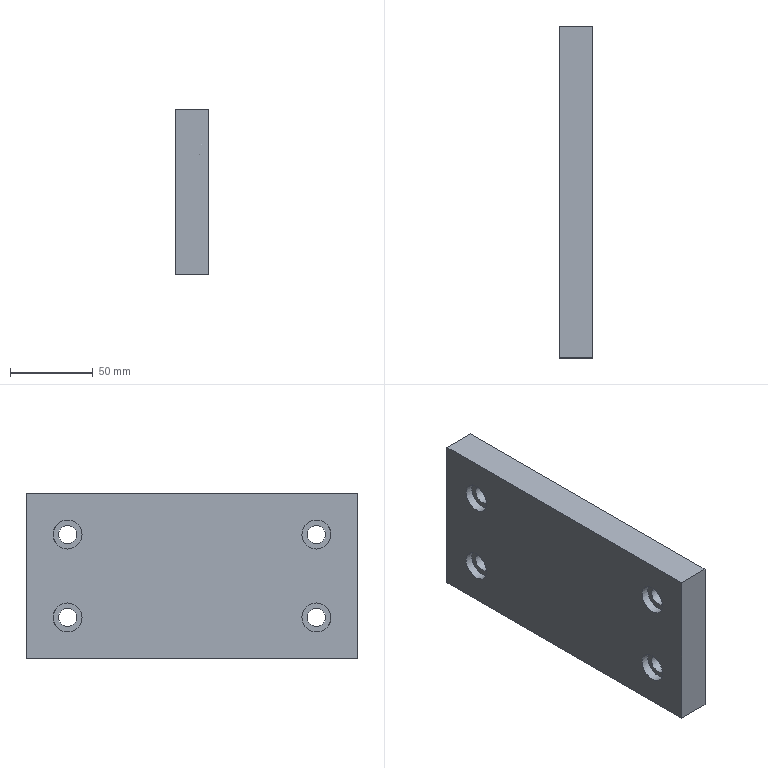Part | NX | features solid 2 | 1 solid | 18 faces | box 20 x 200 x 100 mm | volume 389487 mm3 | plane 10 | cylinder 8 | commonest cylinder face diameters 11 x4 17.5 x4
STEP:
#1=CARTESIAN_POINT('',(-605.,715.,-162.));
#2=VERTEX_POINT('',#1);
#3=CARTESIAN_POINT('',(-605.,715.,-262.));
#4=VERTEX_POINT('',#3);
#5=CARTESIAN_POINT('',(-605.,715.,-160.));
#6=DIRECTION('',(0.,0.,-1.));
#7=VECTOR('',#6,1000.);
#8=LINE('',#5,#7);
#9=EDGE_CURVE('',#2,#4,#8,.T.);
#10=ORIENTED_EDGE('',*,*,#9,.F.);
#11=CARTESIAN_POINT('',(-625.,715.,-162.));
#12=VERTEX_POINT('',#11);
#13=CARTESIAN_POINT('',(-615.,715.,-162.));
#14=DIRECTION('',(1.,0.,0.));
#15=VECTOR('',#14,1000.);
#16=LINE('',#13,#15);
#17=EDGE_CURVE('',#12,#2,#16,.T.);
#18=ORIENTED_EDGE('',*,*,#17,.F.);
#19=CARTESIAN_POINT('',(-625.,715.,-262.));
#20=VERTEX_POINT('',#19);
#21=CARTESIAN_POINT('',(-625.,715.,-160.));
#22=DIRECTION('',(0.,0.,1.));
#23=VECTOR('',#22,1000.);
#24=LINE('',#21,#23);
#25=EDGE_CURVE('',#20,#12,#24,.T.);
#26=ORIENTED_EDGE('',*,*,#25,.F.);
#27=CARTESIAN_POINT('',(-615.,715.,-262.));
#28=DIRECTION('',(1.,0.,0.));
#29=VECTOR('',#28,1000.);
#30=LINE('',#27,#29);
#31=EDGE_CURVE('',#20,#4,#30,.T.);
#32=ORIENTED_EDGE('',*,*,#31,.T.);
#33=EDGE_LOOP('',(#10,#18,#26,#32));
#34=FACE_BOUND('',#33,.T.);
#35=CARTESIAN_POINT('',(-615.,715.,-160.));
#36=DIRECTION('',(0.,-1.,0.));
#37=DIRECTION('',(-1.,0.,0.));
#38=AXIS2_PLACEMENT_3D('',#35,#36,#37);
#39=PLANE('',#38);
#40=ADVANCED_FACE('',(#34),#39,.T.);
#41=CARTESIAN_POINT('',(-605.,740.,-192.5));
#42=VERTEX_POINT('',#41);
#43=CARTESIAN_POINT('',(-605.,740.,-187.));
#44=DIRECTION('',(1.,0.,0.));
#45=DIRECTION('',(0.,0.,-1.));
#46=AXIS2_PLACEMENT_3D('',#43,#44,#45);
#47=CIRCLE('',#46,5.5);
#48=EDGE_CURVE('',#42,#42,#47,.F.);
#49=ORIENTED_EDGE('',*,*,#48,.T.);
#50=EDGE_LOOP('',(#49));
#51=FACE_BOUND('',#50,.T.);
#52=CARTESIAN_POINT('',(-605.,890.,-192.5));
#53=VERTEX_POINT('',#52);
#54=CARTESIAN_POINT('',(-605.,890.,-187.));
#55=DIRECTION('',(1.,0.,0.));
#56=DIRECTION('',(0.,0.,-1.));
#57=AXIS2_PLACEMENT_3D('',#54,#55,#56);
#58=CIRCLE('',#57,5.5);
#59=EDGE_CURVE('',#53,#53,#58,.F.);
#60=ORIENTED_EDGE('',*,*,#59,.T.);
#61=EDGE_LOOP('',(#60));
#62=FACE_BOUND('',#61,.T.);
#63=CARTESIAN_POINT('',(-605.,915.,-262.));
#64=VERTEX_POINT('',#63);
#65=CARTESIAN_POINT('',(-605.,915.,-162.));
#66=VERTEX_POINT('',#65);
#67=CARTESIAN_POINT('',(-605.,915.,-160.));
#68=DIRECTION('',(0.,0.,1.));
#69=VECTOR('',#68,1000.);
#70=LINE('',#67,#69);
#71=EDGE_CURVE('',#64,#66,#70,.T.);
#72=ORIENTED_EDGE('',*,*,#71,.T.);
#73=CARTESIAN_POINT('',(-605.,890.,-162.));
#74=DIRECTION('',(0.,1.,0.));
#75=VECTOR('',#74,1000.);
#76=LINE('',#73,#75);
#77=EDGE_CURVE('',#2,#66,#76,.T.);
#78=ORIENTED_EDGE('',*,*,#77,.F.);
#79=ORIENTED_EDGE('',*,*,#9,.T.);
#80=CARTESIAN_POINT('',(-605.,890.,-262.));
#81=DIRECTION('',(0.,1.,0.));
#82=VECTOR('',#81,1000.);
#83=LINE('',#80,#82);
#84=EDGE_CURVE('',#4,#64,#83,.T.);
#85=ORIENTED_EDGE('',*,*,#84,.T.);
#86=EDGE_LOOP('',(#72,#78,#79,#85));
#87=FACE_BOUND('',#86,.T.);
#88=CARTESIAN_POINT('',(-605.,740.,-231.5));
#89=VERTEX_POINT('',#88);
#90=CARTESIAN_POINT('',(-605.,740.,-237.));
#91=DIRECTION('',(-1.,0.,0.));
#92=DIRECTION('',(0.,0.,1.));
#93=AXIS2_PLACEMENT_3D('',#90,#91,#92);
#94=CIRCLE('',#93,5.5);
#95=EDGE_CURVE('',#89,#89,#94,.F.);
#96=ORIENTED_EDGE('',*,*,#95,.F.);
#97=EDGE_LOOP('',(#96));
#98=FACE_BOUND('',#97,.T.);
#99=CARTESIAN_POINT('',(-605.,890.,-231.5));
#100=VERTEX_POINT('',#99);
#101=CARTESIAN_POINT('',(-605.,890.,-237.));
#102=DIRECTION('',(-1.,0.,0.));
#103=DIRECTION('',(0.,0.,1.));
#104=AXIS2_PLACEMENT_3D('',#101,#102,#103);
#105=CIRCLE('',#104,5.5);
#106=EDGE_CURVE('',#100,#100,#105,.F.);
#107=ORIENTED_EDGE('',*,*,#106,.F.);
#108=EDGE_LOOP('',(#107));
#109=FACE_BOUND('',#108,.T.);
#110=CARTESIAN_POINT('',(-605.,890.,-160.));
#111=DIRECTION('',(1.,0.,0.));
#112=DIRECTION('',(0.,-1.,0.));
#113=AXIS2_PLACEMENT_3D('',#110,#111,#112);
#114=PLANE('',#113);
#115=ADVANCED_FACE('',(#51,#62,#87,#98,#109),#114,.T.);
#116=CARTESIAN_POINT('',(-625.,915.,-162.));
#117=VERTEX_POINT('',#116);
#118=CARTESIAN_POINT('',(-625.,915.,-262.));
#119=VERTEX_POINT('',#118);
#120=CARTESIAN_POINT('',(-625.,915.,-160.));
#121=DIRECTION('',(0.,0.,-1.));
#122=VECTOR('',#121,1000.);
#123=LINE('',#120,#122);
#124=EDGE_CURVE('',#117,#119,#123,.T.);
#125=ORIENTED_EDGE('',*,*,#124,.F.);
#126=CARTESIAN_POINT('',(-615.,915.,-162.));
#127=DIRECTION('',(-1.,0.,0.));
#128=VECTOR('',#127,1000.);
#129=LINE('',#126,#128);
#130=EDGE_CURVE('',#66,#117,#129,.T.);
#131=ORIENTED_EDGE('',*,*,#130,.F.);
#132=ORIENTED_EDGE('',*,*,#71,.F.);
#133=CARTESIAN_POINT('',(-615.,915.,-262.));
#134=DIRECTION('',(-1.,0.,0.));
#135=VECTOR('',#134,1000.);
#136=LINE('',#133,#135);
#137=EDGE_CURVE('',#64,#119,#136,.T.);
#138=ORIENTED_EDGE('',*,*,#137,.T.);
#139=EDGE_LOOP('',(#125,#131,#132,#138));
#140=FACE_BOUND('',#139,.T.);
#141=CARTESIAN_POINT('',(-615.,915.,-160.));
#142=DIRECTION('',(0.,1.,0.));
#143=DIRECTION('',(1.,0.,0.));
#144=AXIS2_PLACEMENT_3D('',#141,#142,#143);
#145=PLANE('',#144);
#146=ADVANCED_FACE('',(#140),#145,.T.);
#147=CARTESIAN_POINT('',(-625.,731.25,-187.));
#148=VERTEX_POINT('',#147);
#149=CARTESIAN_POINT('',(-625.,740.,-187.));
#150=DIRECTION('',(1.,0.,0.));
#151=DIRECTION('',(0.,-1.,0.));
#152=AXIS2_PLACEMENT_3D('',#149,#150,#151);
#153=CIRCLE('',#152,8.75);
#154=EDGE_CURVE('',#148,#148,#153,.T.);
#155=ORIENTED_EDGE('',*,*,#154,.T.);
#156=EDGE_LOOP('',(#155));
#157=FACE_BOUND('',#156,.T.);
#158=CARTESIAN_POINT('',(-625.,881.25,-187.));
#159=VERTEX_POINT('',#158);
#160=CARTESIAN_POINT('',(-625.,890.,-187.));
#161=DIRECTION('',(1.,0.,0.));
#162=DIRECTION('',(0.,-1.,0.));
#163=AXIS2_PLACEMENT_3D('',#160,#161,#162);
#164=CIRCLE('',#163,8.75);
#165=EDGE_CURVE('',#159,#159,#164,.T.);
#166=ORIENTED_EDGE('',*,*,#165,.T.);
#167=EDGE_LOOP('',(#166));
#168=FACE_BOUND('',#167,.T.);
#169=ORIENTED_EDGE('',*,*,#25,.T.);
#170=CARTESIAN_POINT('',(-625.,890.,-162.));
#171=DIRECTION('',(0.,-1.,0.));
#172=VECTOR('',#171,1000.);
#173=LINE('',#170,#172);
#174=EDGE_CURVE('',#117,#12,#173,.T.);
#175=ORIENTED_EDGE('',*,*,#174,.F.);
#176=ORIENTED_EDGE('',*,*,#124,.T.);
#177=CARTESIAN_POINT('',(-625.,890.,-262.));
#178=DIRECTION('',(0.,-1.,0.));
#179=VECTOR('',#178,1000.);
#180=LINE('',#177,#179);
#181=EDGE_CURVE('',#119,#20,#180,.T.);
#182=ORIENTED_EDGE('',*,*,#181,.T.);
#183=EDGE_LOOP('',(#169,#175,#176,#182));
#184=FACE_BOUND('',#183,.T.);
#185=CARTESIAN_POINT('',(-625.,731.25,-237.));
#186=VERTEX_POINT('',#185);
#187=CARTESIAN_POINT('',(-625.,740.,-237.));
#188=DIRECTION('',(-1.,0.,0.));
#189=DIRECTION('',(0.,-1.,0.));
#190=AXIS2_PLACEMENT_3D('',#187,#188,#189);
#191=CIRCLE('',#190,8.75);
#192=EDGE_CURVE('',#186,#186,#191,.T.);
#193=ORIENTED_EDGE('',*,*,#192,.F.);
#194=EDGE_LOOP('',(#193));
#195=FACE_BOUND('',#194,.T.);
#196=CARTESIAN_POINT('',(-625.,881.25,-237.));
#197=VERTEX_POINT('',#196);
#198=CARTESIAN_POINT('',(-625.,890.,-237.));
#199=DIRECTION('',(-1.,0.,0.));
#200=DIRECTION('',(0.,-1.,0.));
#201=AXIS2_PLACEMENT_3D('',#198,#199,#200);
#202=CIRCLE('',#201,8.75);
#203=EDGE_CURVE('',#197,#197,#202,.T.);
#204=ORIENTED_EDGE('',*,*,#203,.F.);
#205=EDGE_LOOP('',(#204));
#206=FACE_BOUND('',#205,.T.);
#207=CARTESIAN_POINT('',(-625.,890.,-160.));
#208=DIRECTION('',(-1.,0.,0.));
#209=DIRECTION('',(0.,1.,0.));
#210=AXIS2_PLACEMENT_3D('',#207,#208,#209);
#211=PLANE('',#210);
#212=ADVANCED_FACE('',(#157,#168,#184,#195,#206),#211,.T.);
#213=CARTESIAN_POINT('',(-620.,740.,-192.5));
#214=VERTEX_POINT('',#213);
#215=CARTESIAN_POINT('',(-620.,740.,-187.));
#216=DIRECTION('',(1.,0.,0.));
#217=DIRECTION('',(0.,0.,-1.));
#218=AXIS2_PLACEMENT_3D('',#215,#216,#217);
#219=CIRCLE('',#218,5.5);
#220=EDGE_CURVE('',#214,#214,#219,.F.);
#221=ORIENTED_EDGE('',*,*,#220,.T.);
#222=EDGE_LOOP('',(#221));
#223=FACE_BOUND('',#222,.T.);
#224=ORIENTED_EDGE('',*,*,#48,.F.);
#225=EDGE_LOOP('',(#224));
#226=FACE_BOUND('',#225,.T.);
#227=CARTESIAN_POINT('',(-605.,740.,-187.));
#228=DIRECTION('',(-1.,0.,0.));
#229=DIRECTION('',(0.,1.,0.));
#230=AXIS2_PLACEMENT_3D('',#227,#228,#229);
#231=CYLINDRICAL_SURFACE('',#230,5.5);
#232=ADVANCED_FACE('',(#223,#226),#231,.F.);
#233=CARTESIAN_POINT('',(-620.,740.,-195.75));
#234=VERTEX_POINT('',#233);
#235=CARTESIAN_POINT('',(-620.,740.,-187.));
#236=DIRECTION('',(1.,0.,0.));
#237=DIRECTION('',(0.,0.,-1.));
#238=AXIS2_PLACEMENT_3D('',#235,#236,#237);
#239=CIRCLE('',#238,8.75);
#240=EDGE_CURVE('',#234,#234,#239,.F.);
#241=ORIENTED_EDGE('',*,*,#240,.T.);
#242=EDGE_LOOP('',(#241));
#243=FACE_BOUND('',#242,.T.);
#244=ORIENTED_EDGE('',*,*,#220,.F.);
#245=EDGE_LOOP('',(#244));
#246=FACE_BOUND('',#245,.T.);
#247=CARTESIAN_POINT('',(-620.,740.,-187.));
#248=DIRECTION('',(1.,0.,0.));
#249=DIRECTION('',(0.,-1.,0.));
#250=AXIS2_PLACEMENT_3D('',#247,#248,#249);
#251=PLANE('',#250);
#252=ADVANCED_FACE('',(#243,#246),#251,.F.);
#253=ORIENTED_EDGE('',*,*,#154,.F.);
#254=EDGE_LOOP('',(#253));
#255=FACE_BOUND('',#254,.T.);
#256=ORIENTED_EDGE('',*,*,#240,.F.);
#257=EDGE_LOOP('',(#256));
#258=FACE_BOUND('',#257,.T.);
#259=CARTESIAN_POINT('',(-610.,740.,-187.));
#260=DIRECTION('',(-1.,0.,0.));
#261=DIRECTION('',(0.,1.,0.));
#262=AXIS2_PLACEMENT_3D('',#259,#260,#261);
#263=CYLINDRICAL_SURFACE('',#262,8.75);
#264=ADVANCED_FACE('',(#255,#258),#263,.F.);
#265=CARTESIAN_POINT('',(-620.,890.,-192.5));
#266=VERTEX_POINT('',#265);
#267=CARTESIAN_POINT('',(-620.,890.,-187.));
#268=DIRECTION('',(1.,0.,0.));
#269=DIRECTION('',(0.,0.,-1.));
#270=AXIS2_PLACEMENT_3D('',#267,#268,#269);
#271=CIRCLE('',#270,5.5);
#272=EDGE_CURVE('',#266,#266,#271,.F.);
#273=ORIENTED_EDGE('',*,*,#272,.T.);
#274=EDGE_LOOP('',(#273));
#275=FACE_BOUND('',#274,.T.);
#276=ORIENTED_EDGE('',*,*,#59,.F.);
#277=EDGE_LOOP('',(#276));
#278=FACE_BOUND('',#277,.T.);
#279=CARTESIAN_POINT('',(-605.,890.,-187.));
#280=DIRECTION('',(-1.,0.,0.));
#281=DIRECTION('',(0.,1.,0.));
#282=AXIS2_PLACEMENT_3D('',#279,#280,#281);
#283=CYLINDRICAL_SURFACE('',#282,5.5);
#284=ADVANCED_FACE('',(#275,#278),#283,.F.);
#285=CARTESIAN_POINT('',(-620.,890.,-195.75));
#286=VERTEX_POINT('',#285);
#287=CARTESIAN_POINT('',(-620.,890.,-187.));
#288=DIRECTION('',(1.,0.,0.));
#289=DIRECTION('',(0.,0.,-1.));
#290=AXIS2_PLACEMENT_3D('',#287,#288,#289);
#291=CIRCLE('',#290,8.75);
#292=EDGE_CURVE('',#286,#286,#291,.F.);
#293=ORIENTED_EDGE('',*,*,#292,.T.);
#294=EDGE_LOOP('',(#293));
#295=FACE_BOUND('',#294,.T.);
#296=ORIENTED_EDGE('',*,*,#272,.F.);
#297=EDGE_LOOP('',(#296));
#298=FACE_BOUND('',#297,.T.);
#299=CARTESIAN_POINT('',(-620.,890.,-187.));
#300=DIRECTION('',(1.,0.,0.));
#301=DIRECTION('',(0.,-1.,0.));
#302=AXIS2_PLACEMENT_3D('',#299,#300,#301);
#303=PLANE('',#302);
#304=ADVANCED_FACE('',(#295,#298),#303,.F.);
#305=ORIENTED_EDGE('',*,*,#165,.F.);
#306=EDGE_LOOP('',(#305));
#307=FACE_BOUND('',#306,.T.);
#308=ORIENTED_EDGE('',*,*,#292,.F.);
#309=EDGE_LOOP('',(#308));
#310=FACE_BOUND('',#309,.T.);
#311=CARTESIAN_POINT('',(-610.,890.,-187.));
#312=DIRECTION('',(-1.,0.,0.));
#313=DIRECTION('',(0.,1.,0.));
#314=AXIS2_PLACEMENT_3D('',#311,#312,#313);
#315=CYLINDRICAL_SURFACE('',#314,8.75);
#316=ADVANCED_FACE('',(#307,#310),#315,.F.);
#317=ORIENTED_EDGE('',*,*,#17,.T.);
#318=ORIENTED_EDGE('',*,*,#77,.T.);
#319=ORIENTED_EDGE('',*,*,#130,.T.);
#320=ORIENTED_EDGE('',*,*,#174,.T.);
#321=EDGE_LOOP('',(#317,#318,#319,#320));
#322=FACE_BOUND('',#321,.T.);
#323=CARTESIAN_POINT('',(-605.,640.,-162.));
#324=DIRECTION('',(0.,0.,-1.));
#325=DIRECTION('',(-1.,0.,0.));
#326=AXIS2_PLACEMENT_3D('',#323,#324,#325);
#327=PLANE('',#326);
#328=ADVANCED_FACE('',(#322),#327,.F.);
#329=CARTESIAN_POINT('',(-620.,740.,-231.5));
#330=VERTEX_POINT('',#329);
#331=CARTESIAN_POINT('',(-620.,740.,-237.));
#332=DIRECTION('',(-1.,0.,0.));
#333=DIRECTION('',(0.,0.,1.));
#334=AXIS2_PLACEMENT_3D('',#331,#332,#333);
#335=CIRCLE('',#334,5.5);
#336=EDGE_CURVE('',#330,#330,#335,.F.);
#337=ORIENTED_EDGE('',*,*,#336,.F.);
#338=EDGE_LOOP('',(#337));
#339=FACE_BOUND('',#338,.T.);
#340=ORIENTED_EDGE('',*,*,#95,.T.);
#341=EDGE_LOOP('',(#340));
#342=FACE_BOUND('',#341,.T.);
#343=CARTESIAN_POINT('',(-605.,740.,-237.));
#344=DIRECTION('',(-1.,0.,0.));
#345=DIRECTION('',(0.,1.,0.));
#346=AXIS2_PLACEMENT_3D('',#343,#344,#345);
#347=CYLINDRICAL_SURFACE('',#346,5.5);
#348=ADVANCED_FACE('',(#339,#342),#347,.F.);
#349=CARTESIAN_POINT('',(-620.,740.,-228.25));
#350=VERTEX_POINT('',#349);
#351=CARTESIAN_POINT('',(-620.,740.,-237.));
#352=DIRECTION('',(-1.,0.,0.));
#353=DIRECTION('',(0.,0.,1.));
#354=AXIS2_PLACEMENT_3D('',#351,#352,#353);
#355=CIRCLE('',#354,8.75);
#356=EDGE_CURVE('',#350,#350,#355,.F.);
#357=ORIENTED_EDGE('',*,*,#356,.F.);
#358=EDGE_LOOP('',(#357));
#359=FACE_BOUND('',#358,.T.);
#360=ORIENTED_EDGE('',*,*,#336,.T.);
#361=EDGE_LOOP('',(#360));
#362=FACE_BOUND('',#361,.T.);
#363=CARTESIAN_POINT('',(-620.,740.,-237.));
#364=DIRECTION('',(1.,0.,0.));
#365=DIRECTION('',(0.,-1.,0.));
#366=AXIS2_PLACEMENT_3D('',#363,#364,#365);
#367=PLANE('',#366);
#368=ADVANCED_FACE('',(#359,#362),#367,.F.);
#369=ORIENTED_EDGE('',*,*,#192,.T.);
#370=EDGE_LOOP('',(#369));
#371=FACE_BOUND('',#370,.T.);
#372=ORIENTED_EDGE('',*,*,#356,.T.);
#373=EDGE_LOOP('',(#372));
#374=FACE_BOUND('',#373,.T.);
#375=CARTESIAN_POINT('',(-610.,740.,-237.));
#376=DIRECTION('',(-1.,0.,0.));
#377=DIRECTION('',(0.,1.,0.));
#378=AXIS2_PLACEMENT_3D('',#375,#376,#377);
#379=CYLINDRICAL_SURFACE('',#378,8.75);
#380=ADVANCED_FACE('',(#371,#374),#379,.F.);
#381=CARTESIAN_POINT('',(-620.,890.,-231.5));
#382=VERTEX_POINT('',#381);
#383=CARTESIAN_POINT('',(-620.,890.,-237.));
#384=DIRECTION('',(-1.,0.,0.));
#385=DIRECTION('',(0.,0.,1.));
#386=AXIS2_PLACEMENT_3D('',#383,#384,#385);
#387=CIRCLE('',#386,5.5);
#388=EDGE_CURVE('',#382,#382,#387,.F.);
#389=ORIENTED_EDGE('',*,*,#388,.F.);
#390=EDGE_LOOP('',(#389));
#391=FACE_BOUND('',#390,.T.);
#392=ORIENTED_EDGE('',*,*,#106,.T.);
#393=EDGE_LOOP('',(#392));
#394=FACE_BOUND('',#393,.T.);
#395=CARTESIAN_POINT('',(-605.,890.,-237.));
#396=DIRECTION('',(-1.,0.,0.));
#397=DIRECTION('',(0.,1.,0.));
#398=AXIS2_PLACEMENT_3D('',#395,#396,#397);
#399=CYLINDRICAL_SURFACE('',#398,5.5);
#400=ADVANCED_FACE('',(#391,#394),#399,.F.);
#401=CARTESIAN_POINT('',(-620.,890.,-228.25));
#402=VERTEX_POINT('',#401);
#403=CARTESIAN_POINT('',(-620.,890.,-237.));
#404=DIRECTION('',(-1.,0.,0.));
#405=DIRECTION('',(0.,0.,1.));
#406=AXIS2_PLACEMENT_3D('',#403,#404,#405);
#407=CIRCLE('',#406,8.75);
#408=EDGE_CURVE('',#402,#402,#407,.F.);
#409=ORIENTED_EDGE('',*,*,#408,.F.);
#410=EDGE_LOOP('',(#409));
#411=FACE_BOUND('',#410,.T.);
#412=ORIENTED_EDGE('',*,*,#388,.T.);
#413=EDGE_LOOP('',(#412));
#414=FACE_BOUND('',#413,.T.);
#415=CARTESIAN_POINT('',(-620.,890.,-237.));
#416=DIRECTION('',(1.,0.,0.));
#417=DIRECTION('',(0.,-1.,0.));
#418=AXIS2_PLACEMENT_3D('',#415,#416,#417);
#419=PLANE('',#418);
#420=ADVANCED_FACE('',(#411,#414),#419,.F.);
#421=ORIENTED_EDGE('',*,*,#203,.T.);
#422=EDGE_LOOP('',(#421));
#423=FACE_BOUND('',#422,.T.);
#424=ORIENTED_EDGE('',*,*,#408,.T.);
#425=EDGE_LOOP('',(#424));
#426=FACE_BOUND('',#425,.T.);
#427=CARTESIAN_POINT('',(-610.,890.,-237.));
#428=DIRECTION('',(-1.,0.,0.));
#429=DIRECTION('',(0.,1.,0.));
#430=AXIS2_PLACEMENT_3D('',#427,#428,#429);
#431=CYLINDRICAL_SURFACE('',#430,8.75);
#432=ADVANCED_FACE('',(#423,#426),#431,.F.);
#433=ORIENTED_EDGE('',*,*,#31,.F.);
#434=ORIENTED_EDGE('',*,*,#181,.F.);
#435=ORIENTED_EDGE('',*,*,#137,.F.);
#436=ORIENTED_EDGE('',*,*,#84,.F.);
#437=EDGE_LOOP('',(#433,#434,#435,#436));
#438=FACE_BOUND('',#437,.T.);
#439=CARTESIAN_POINT('',(-605.,640.,-262.));
#440=DIRECTION('',(0.,0.,1.));
#441=DIRECTION('',(-1.,0.,0.));
#442=AXIS2_PLACEMENT_3D('',#439,#440,#441);
#443=PLANE('',#442);
#444=ADVANCED_FACE('',(#438),#443,.F.);
#445=CLOSED_SHELL('',(#40,#115,#146,#212,#232,#252,#264,#284,#304,#316,#328,#348,#368,#380,#400,#420,#432,#444));
#446=MANIFOLD_SOLID_BREP('',#445);
#447=(LENGTH_UNIT()NAMED_UNIT(*)SI_UNIT(.MILLI.,.METRE.));
#448=UNCERTAINTY_MEASURE_WITH_UNIT(LENGTH_MEASURE(0.00001),#447,'','');
#449=(NAMED_UNIT(*)PLANE_ANGLE_UNIT()SI_UNIT($,.RADIAN.));
#450=(NAMED_UNIT(*)SI_UNIT($,.STERADIAN.)SOLID_ANGLE_UNIT());
#451=(GEOMETRIC_REPRESENTATION_CONTEXT(3)GLOBAL_UNCERTAINTY_ASSIGNED_CONTEXT((#448))GLOBAL_UNIT_ASSIGNED_CONTEXT((#447,#449,#450))REPRESENTATION_CONTEXT('',''));
#452=ADVANCED_BREP_SHAPE_REPRESENTATION('',(#446),#451);